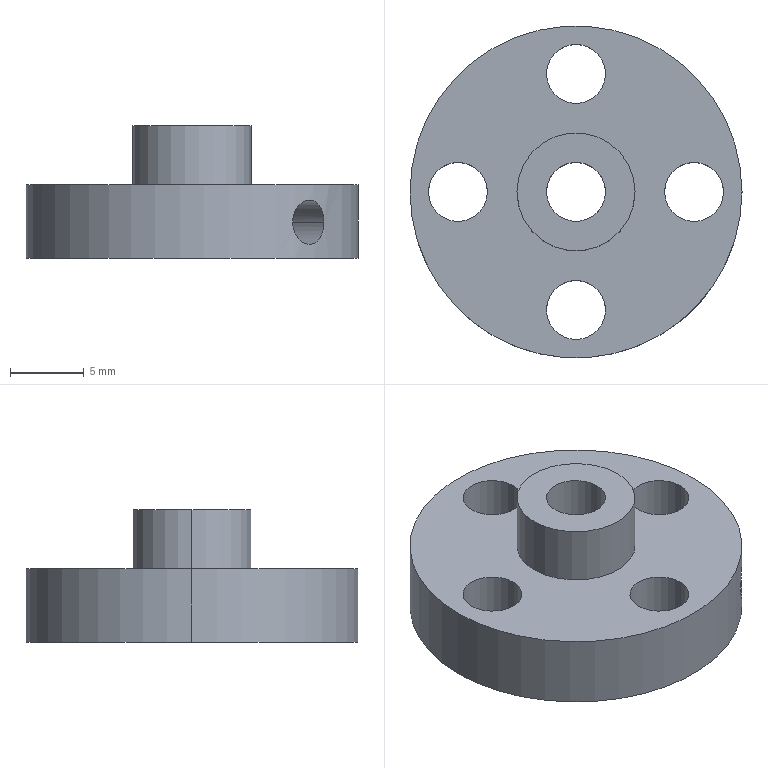Part | SolidWorks | features ICE 2, Extrusion 1 | 1 solid | 19 faces | box 22.5 x 22.5 x 9 mm | volume 1758 mm3 | cylinder 16 | plane 3 | commonest cylinder face diameters 4 x10 3 x2 8 x2 22.5 x2
STEP:
#1=CARTESIAN_POINT('',(2.,0.,1.958));
#2=VERTEX_POINT('',#1);
#3=CARTESIAN_POINT('',(-0.1252,-1.996,2.458));
#4=VERTEX_POINT('',#3);
#5=CARTESIAN_POINT('',(2.,0.,1.958));
#6=CARTESIAN_POINT('',(2.,-0.08244,1.793));
#7=CARTESIAN_POINT('',(1.995,-0.1967,1.645));
#8=CARTESIAN_POINT('',(1.952,-0.4524,1.385));
#9=CARTESIAN_POINT('',(1.915,-0.5972,1.271));
#10=CARTESIAN_POINT('',(1.797,-0.8915,1.091));
#11=CARTESIAN_POINT('',(1.714,-1.047,1.023));
#12=CARTESIAN_POINT('',(1.553,-1.264,0.9695));
#13=CARTESIAN_POINT('',(1.492,-1.335,0.9596));
#14=CARTESIAN_POINT('',(1.363,-1.466,0.9573));
#15=CARTESIAN_POINT('',(1.295,-1.527,0.9646));
#16=CARTESIAN_POINT('',(1.078,-1.694,1.011));
#17=CARTESIAN_POINT('',(0.9236,-1.781,1.075));
#18=CARTESIAN_POINT('',(0.6239,-1.907,1.251));
#19=CARTESIAN_POINT('',(0.4783,-1.946,1.363));
#20=CARTESIAN_POINT('',(0.2185,-1.992,1.619));
#21=CARTESIAN_POINT('',(0.1016,-1.999,1.766));
#22=CARTESIAN_POINT('',(-0.07068,-2.001,2.091));
#23=CARTESIAN_POINT('',(-0.1252,-1.996,2.273));
#24=CARTESIAN_POINT('',(-0.1252,-1.996,2.458));
#25=B_SPLINE_CURVE_WITH_KNOTS('',3,(#5,#6,#7,#8,#9,#10,#11,#12,#13,#14,#15,#16,#17,#18,#19,#20,#21,#22,#23,#24),.UNSPECIFIED.,.F.,.F.,(4,2,2,2,2,2,2,2,2,4),(0.0005162,0.001064,0.001612,0.00216,0.002434,0.002708,0.003256,0.003804,0.004352,0.004899),.UNSPECIFIED.);
#26=EDGE_CURVE('',#2,#4,#25,.T.);
#27=ORIENTED_EDGE('',*,*,#26,.T.);
#28=CARTESIAN_POINT('',(6.823,-8.945,2.458));
#29=VERTEX_POINT('',#28);
#30=CARTESIAN_POINT('',(-0.1768,-1.945,2.458));
#31=DIRECTION('',(0.7071,-0.7071,0.));
#32=VECTOR('',#31,1000.);
#33=LINE('',#30,#32);
#34=EDGE_CURVE('',#4,#29,#33,.T.);
#35=ORIENTED_EDGE('',*,*,#34,.T.);
#36=CARTESIAN_POINT('',(8.945,-6.823,2.458));
#37=VERTEX_POINT('',#36);
#38=CARTESIAN_POINT('',(8.945,-6.823,2.458));
#39=CARTESIAN_POINT('',(8.945,-6.823,2.359));
#40=CARTESIAN_POINT('',(8.939,-6.831,2.262));
#41=CARTESIAN_POINT('',(8.915,-6.862,2.07));
#42=CARTESIAN_POINT('',(8.897,-6.885,1.974));
#43=CARTESIAN_POINT('',(8.851,-6.945,1.793));
#44=CARTESIAN_POINT('',(8.822,-6.981,1.707));
#45=CARTESIAN_POINT('',(8.754,-7.067,1.544));
#46=CARTESIAN_POINT('',(8.714,-7.116,1.467));
#47=CARTESIAN_POINT('',(8.581,-7.277,1.259));
#48=CARTESIAN_POINT('',(8.472,-7.404,1.148));
#49=CARTESIAN_POINT('',(8.23,-7.672,0.9979));
#50=CARTESIAN_POINT('',(8.094,-7.816,0.9584));
#51=CARTESIAN_POINT('',(7.886,-8.024,0.9583));
#52=CARTESIAN_POINT('',(7.815,-8.093,0.9681));
#53=CARTESIAN_POINT('',(7.675,-8.226,1.006));
#54=CARTESIAN_POINT('',(7.606,-8.289,1.035));
#55=CARTESIAN_POINT('',(7.404,-8.472,1.148));
#56=CARTESIAN_POINT('',(7.278,-8.58,1.258));
#57=CARTESIAN_POINT('',(7.115,-8.714,1.468));
#58=CARTESIAN_POINT('',(7.067,-8.753,1.543));
#59=CARTESIAN_POINT('',(6.982,-8.822,1.706));
#60=CARTESIAN_POINT('',(6.944,-8.851,1.793));
#61=CARTESIAN_POINT('',(6.885,-8.898,1.975));
#62=CARTESIAN_POINT('',(6.862,-8.915,2.068));
#63=CARTESIAN_POINT('',(6.831,-8.939,2.261));
#64=CARTESIAN_POINT('',(6.823,-8.945,2.36));
#65=CARTESIAN_POINT('',(6.823,-8.945,2.458));
#66=B_SPLINE_CURVE_WITH_KNOTS('',3,(#38,#39,#40,#41,#42,#43,#44,#45,#46,#47,#48,#49,#50,#51,#52,#53,#54,#55,#56,#57,#58,#59,#60,#61,#62,#63,#64,#65),.UNSPECIFIED.,.F.,.F.,(4,2,2,2,2,2,2,2,2,2,2,2,2,4),(0.,0.0002934,0.0005869,0.0008803,0.001174,0.001761,0.002347,0.002641,0.002934,0.003521,0.003815,0.004108,0.004401,0.004695),.UNSPECIFIED.);
#67=EDGE_CURVE('',#37,#29,#66,.T.);
#68=ORIENTED_EDGE('',*,*,#67,.F.);
#69=CARTESIAN_POINT('',(1.996,0.1252,2.458));
#70=VERTEX_POINT('',#69);
#71=CARTESIAN_POINT('',(1.945,0.1768,2.458));
#72=DIRECTION('',(0.7071,-0.7071,0.));
#73=VECTOR('',#72,1000.);
#74=LINE('',#71,#73);
#75=EDGE_CURVE('',#70,#37,#74,.T.);
#76=ORIENTED_EDGE('',*,*,#75,.F.);
#77=CARTESIAN_POINT('',(1.996,0.1252,2.458));
#78=CARTESIAN_POINT('',(1.996,0.1252,2.371));
#79=CARTESIAN_POINT('',(1.997,0.1136,2.285));
#80=CARTESIAN_POINT('',(1.999,0.07067,2.118));
#81=CARTESIAN_POINT('',(2.,0.03884,2.036));
#82=CARTESIAN_POINT('',(2.,0.,1.958));
#83=B_SPLINE_CURVE_WITH_KNOTS('',3,(#77,#78,#79,#80,#81,#82),.UNSPECIFIED.,.F.,.F.,(4,2,4),(0.,0.0002581,0.0005162),.UNSPECIFIED.);
#84=EDGE_CURVE('',#70,#2,#83,.T.);
#85=ORIENTED_EDGE('',*,*,#84,.T.);
#86=EDGE_LOOP('',(#27,#35,#68,#76,#85));
#87=FACE_OUTER_BOUND('',#86,.T.);
#88=CARTESIAN_POINT('',(0.8839,-0.8839,2.458));
#89=DIRECTION('',(0.7071,-0.7071,0.));
#90=DIRECTION('',(0.7071,0.7071,0.));
#91=AXIS2_PLACEMENT_3D('',#88,#89,#90);
#92=CYLINDRICAL_SURFACE('',#91,1.5);
#93=ADVANCED_FACE('',(#87),#92,.F.);
#94=CARTESIAN_POINT('',(4.,0.,9.));
#95=VERTEX_POINT('',#94);
#96=CARTESIAN_POINT('',(-4.,0.,9.));
#97=VERTEX_POINT('',#96);
#98=CARTESIAN_POINT('',(0.,0.,9.));
#99=DIRECTION('',(0.,0.,1.));
#100=DIRECTION('',(1.,0.,0.));
#101=AXIS2_PLACEMENT_3D('',#98,#99,#100);
#102=CIRCLE('',#101,4.);
#103=EDGE_CURVE('',#95,#97,#102,.T.);
#104=ORIENTED_EDGE('',*,*,#103,.F.);
#105=CARTESIAN_POINT('',(4.,0.,5.));
#106=VERTEX_POINT('',#105);
#107=CARTESIAN_POINT('',(4.,0.,9.));
#108=DIRECTION('',(0.,0.,-1.));
#109=VECTOR('',#108,1000.);
#110=LINE('',#107,#109);
#111=EDGE_CURVE('',#95,#106,#110,.T.);
#112=ORIENTED_EDGE('',*,*,#111,.T.);
#113=CARTESIAN_POINT('',(-4.,0.,5.));
#114=VERTEX_POINT('',#113);
#115=CARTESIAN_POINT('',(0.,0.,5.));
#116=DIRECTION('',(0.,0.,1.));
#117=DIRECTION('',(1.,0.,0.));
#118=AXIS2_PLACEMENT_3D('',#115,#116,#117);
#119=CIRCLE('',#118,4.);
#120=EDGE_CURVE('',#106,#114,#119,.T.);
#121=ORIENTED_EDGE('',*,*,#120,.T.);
#122=CARTESIAN_POINT('',(-4.,0.,9.));
#123=DIRECTION('',(0.,0.,-1.));
#124=VECTOR('',#123,1000.);
#125=LINE('',#122,#124);
#126=EDGE_CURVE('',#97,#114,#125,.T.);
#127=ORIENTED_EDGE('',*,*,#126,.F.);
#128=EDGE_LOOP('',(#104,#112,#121,#127));
#129=FACE_OUTER_BOUND('',#128,.T.);
#130=CARTESIAN_POINT('',(0.,0.,9.));
#131=DIRECTION('',(0.,0.,-1.));
#132=DIRECTION('',(-1.,0.,0.));
#133=AXIS2_PLACEMENT_3D('',#130,#131,#132);
#134=CYLINDRICAL_SURFACE('',#133,4.);
#135=ADVANCED_FACE('',(#129),#134,.T.);
#136=CARTESIAN_POINT('',(6.,0.,5.));
#137=VERTEX_POINT('',#136);
#138=CARTESIAN_POINT('',(10.,0.,5.));
#139=VERTEX_POINT('',#138);
#140=CARTESIAN_POINT('',(8.,0.,5.));
#141=DIRECTION('',(0.,0.,1.));
#142=DIRECTION('',(1.,0.,0.));
#143=AXIS2_PLACEMENT_3D('',#140,#141,#142);
#144=CIRCLE('',#143,2.);
#145=EDGE_CURVE('',#137,#139,#144,.T.);
#146=ORIENTED_EDGE('',*,*,#145,.T.);
#147=CARTESIAN_POINT('',(10.,0.,0.));
#148=VERTEX_POINT('',#147);
#149=CARTESIAN_POINT('',(10.,0.,5.));
#150=DIRECTION('',(0.,0.,-1.));
#151=VECTOR('',#150,1000.);
#152=LINE('',#149,#151);
#153=EDGE_CURVE('',#139,#148,#152,.T.);
#154=ORIENTED_EDGE('',*,*,#153,.T.);
#155=CARTESIAN_POINT('',(6.,0.,0.));
#156=VERTEX_POINT('',#155);
#157=CARTESIAN_POINT('',(8.,0.,0.));
#158=DIRECTION('',(0.,0.,1.));
#159=DIRECTION('',(1.,0.,0.));
#160=AXIS2_PLACEMENT_3D('',#157,#158,#159);
#161=CIRCLE('',#160,2.);
#162=EDGE_CURVE('',#156,#148,#161,.T.);
#163=ORIENTED_EDGE('',*,*,#162,.F.);
#164=CARTESIAN_POINT('',(6.,0.,5.));
#165=DIRECTION('',(0.,0.,-1.));
#166=VECTOR('',#165,1000.);
#167=LINE('',#164,#166);
#168=EDGE_CURVE('',#137,#156,#167,.T.);
#169=ORIENTED_EDGE('',*,*,#168,.F.);
#170=EDGE_LOOP('',(#146,#154,#163,#169));
#171=FACE_OUTER_BOUND('',#170,.T.);
#172=CARTESIAN_POINT('',(8.,0.,5.));
#173=DIRECTION('',(0.,0.,-1.));
#174=DIRECTION('',(-1.,0.,0.));
#175=AXIS2_PLACEMENT_3D('',#172,#173,#174);
#176=CYLINDRICAL_SURFACE('',#175,2.);
#177=ADVANCED_FACE('',(#171),#176,.F.);
#178=CARTESIAN_POINT('',(-2.,0.,9.));
#179=VERTEX_POINT('',#178);
#180=CARTESIAN_POINT('',(2.,0.,9.));
#181=VERTEX_POINT('',#180);
#182=CARTESIAN_POINT('',(0.,0.,9.));
#183=DIRECTION('',(0.,0.,1.));
#184=DIRECTION('',(1.,0.,0.));
#185=AXIS2_PLACEMENT_3D('',#182,#183,#184);
#186=CIRCLE('',#185,2.);
#187=EDGE_CURVE('',#179,#181,#186,.T.);
#188=ORIENTED_EDGE('',*,*,#187,.T.);
#189=CARTESIAN_POINT('',(2.,0.,2.958));
#190=VERTEX_POINT('',#189);
#191=CARTESIAN_POINT('',(2.,0.,5.));
#192=DIRECTION('',(0.,0.,-1.));
#193=VECTOR('',#192,1000.);
#194=LINE('',#191,#193);
#195=EDGE_CURVE('',#181,#190,#194,.T.);
#196=ORIENTED_EDGE('',*,*,#195,.T.);
#197=CARTESIAN_POINT('',(-0.1252,-1.996,2.458));
#198=CARTESIAN_POINT('',(-0.1252,-1.996,2.644));
#199=CARTESIAN_POINT('',(-0.07048,-2.001,2.826));
#200=CARTESIAN_POINT('',(0.1014,-1.999,3.151));
#201=CARTESIAN_POINT('',(0.2181,-1.992,3.297));
#202=CARTESIAN_POINT('',(0.4776,-1.947,3.553));
#203=CARTESIAN_POINT('',(0.6235,-1.907,3.665));
#204=CARTESIAN_POINT('',(0.9189,-1.784,3.839));
#205=CARTESIAN_POINT('',(1.074,-1.697,3.904));
#206=CARTESIAN_POINT('',(1.289,-1.532,3.951));
#207=CARTESIAN_POINT('',(1.36,-1.47,3.959));
#208=CARTESIAN_POINT('',(1.489,-1.338,3.957));
#209=CARTESIAN_POINT('',(1.548,-1.269,3.948));
#210=CARTESIAN_POINT('',(1.712,-1.05,3.895));
#211=CARTESIAN_POINT('',(1.795,-0.8957,3.828));
#212=CARTESIAN_POINT('',(1.915,-0.5973,3.646));
#213=CARTESIAN_POINT('',(1.952,-0.4528,3.532));
#214=CARTESIAN_POINT('',(1.995,-0.1968,3.272));
#215=CARTESIAN_POINT('',(2.,-0.08225,3.123));
#216=CARTESIAN_POINT('',(2.,0.,2.958));
#217=B_SPLINE_CURVE_WITH_KNOTS('',3,(#197,#198,#199,#200,#201,#202,#203,#204,#205,#206,#207,#208,#209,#210,#211,#212,#213,#214,#215,#216),.UNSPECIFIED.,.F.,.F.,(4,2,2,2,2,2,2,2,2,4),(0.004899,0.005447,0.005994,0.006541,0.007088,0.007362,0.007635,0.008182,0.008729,0.009276),.UNSPECIFIED.);
#218=EDGE_CURVE('',#4,#190,#217,.T.);
#219=ORIENTED_EDGE('',*,*,#218,.F.);
#220=ORIENTED_EDGE('',*,*,#26,.F.);
#221=CARTESIAN_POINT('',(2.,0.,0.));
#222=VERTEX_POINT('',#221);
#223=CARTESIAN_POINT('',(2.,0.,5.));
#224=DIRECTION('',(0.,0.,-1.));
#225=VECTOR('',#224,1000.);
#226=LINE('',#223,#225);
#227=EDGE_CURVE('',#2,#222,#226,.T.);
#228=ORIENTED_EDGE('',*,*,#227,.T.);
#229=CARTESIAN_POINT('',(-2.,0.,0.));
#230=VERTEX_POINT('',#229);
#231=CARTESIAN_POINT('',(0.,0.,0.));
#232=DIRECTION('',(0.,0.,1.));
#233=DIRECTION('',(1.,0.,0.));
#234=AXIS2_PLACEMENT_3D('',#231,#232,#233);
#235=CIRCLE('',#234,2.);
#236=EDGE_CURVE('',#230,#222,#235,.T.);
#237=ORIENTED_EDGE('',*,*,#236,.F.);
#238=CARTESIAN_POINT('',(-2.,0.,5.));
#239=DIRECTION('',(0.,0.,-1.));
#240=VECTOR('',#239,1000.);
#241=LINE('',#238,#240);
#242=EDGE_CURVE('',#179,#230,#241,.T.);
#243=ORIENTED_EDGE('',*,*,#242,.F.);
#244=EDGE_LOOP('',(#188,#196,#219,#220,#228,#237,#243));
#245=FACE_OUTER_BOUND('',#244,.T.);
#246=CARTESIAN_POINT('',(0.,0.,5.));
#247=DIRECTION('',(0.,0.,-1.));
#248=DIRECTION('',(-1.,0.,0.));
#249=AXIS2_PLACEMENT_3D('',#246,#247,#248);
#250=CYLINDRICAL_SURFACE('',#249,2.);
#251=ADVANCED_FACE('',(#245),#250,.F.);
#252=CARTESIAN_POINT('',(-2.,8.,5.));
#253=VERTEX_POINT('',#252);
#254=CARTESIAN_POINT('',(2.,8.,5.));
#255=VERTEX_POINT('',#254);
#256=CARTESIAN_POINT('',(0.,8.,5.));
#257=DIRECTION('',(0.,0.,1.));
#258=DIRECTION('',(1.,0.,0.));
#259=AXIS2_PLACEMENT_3D('',#256,#257,#258);
#260=CIRCLE('',#259,2.);
#261=EDGE_CURVE('',#253,#255,#260,.T.);
#262=ORIENTED_EDGE('',*,*,#261,.T.);
#263=CARTESIAN_POINT('',(2.,8.,0.));
#264=VERTEX_POINT('',#263);
#265=CARTESIAN_POINT('',(2.,8.,5.));
#266=DIRECTION('',(0.,0.,-1.));
#267=VECTOR('',#266,1000.);
#268=LINE('',#265,#267);
#269=EDGE_CURVE('',#255,#264,#268,.T.);
#270=ORIENTED_EDGE('',*,*,#269,.T.);
#271=CARTESIAN_POINT('',(-2.,8.,0.));
#272=VERTEX_POINT('',#271);
#273=CARTESIAN_POINT('',(0.,8.,0.));
#274=DIRECTION('',(0.,0.,1.));
#275=DIRECTION('',(1.,0.,0.));
#276=AXIS2_PLACEMENT_3D('',#273,#274,#275);
#277=CIRCLE('',#276,2.);
#278=EDGE_CURVE('',#272,#264,#277,.T.);
#279=ORIENTED_EDGE('',*,*,#278,.F.);
#280=CARTESIAN_POINT('',(-2.,8.,5.));
#281=DIRECTION('',(0.,0.,-1.));
#282=VECTOR('',#281,1000.);
#283=LINE('',#280,#282);
#284=EDGE_CURVE('',#253,#272,#283,.T.);
#285=ORIENTED_EDGE('',*,*,#284,.F.);
#286=EDGE_LOOP('',(#262,#270,#279,#285));
#287=FACE_OUTER_BOUND('',#286,.T.);
#288=CARTESIAN_POINT('',(0.,8.,5.));
#289=DIRECTION('',(0.,0.,-1.));
#290=DIRECTION('',(-1.,0.,0.));
#291=AXIS2_PLACEMENT_3D('',#288,#289,#290);
#292=CYLINDRICAL_SURFACE('',#291,2.);
#293=ADVANCED_FACE('',(#287),#292,.F.);
#294=CARTESIAN_POINT('',(11.25,0.,5.));
#295=VERTEX_POINT('',#294);
#296=CARTESIAN_POINT('',(-11.25,0.,5.));
#297=VERTEX_POINT('',#296);
#298=CARTESIAN_POINT('',(0.,0.,5.));
#299=DIRECTION('',(0.,0.,1.));
#300=DIRECTION('',(1.,0.,0.));
#301=AXIS2_PLACEMENT_3D('',#298,#299,#300);
#302=CIRCLE('',#301,11.25);
#303=EDGE_CURVE('',#295,#297,#302,.T.);
#304=ORIENTED_EDGE('',*,*,#303,.F.);
#305=CARTESIAN_POINT('',(11.25,0.,0.));
#306=VERTEX_POINT('',#305);
#307=CARTESIAN_POINT('',(11.25,0.,5.));
#308=DIRECTION('',(0.,0.,-1.));
#309=VECTOR('',#308,1000.);
#310=LINE('',#307,#309);
#311=EDGE_CURVE('',#295,#306,#310,.T.);
#312=ORIENTED_EDGE('',*,*,#311,.T.);
#313=CARTESIAN_POINT('',(-11.25,0.,0.));
#314=VERTEX_POINT('',#313);
#315=CARTESIAN_POINT('',(0.,0.,0.));
#316=DIRECTION('',(0.,0.,1.));
#317=DIRECTION('',(1.,0.,0.));
#318=AXIS2_PLACEMENT_3D('',#315,#316,#317);
#319=CIRCLE('',#318,11.25);
#320=EDGE_CURVE('',#306,#314,#319,.T.);
#321=ORIENTED_EDGE('',*,*,#320,.T.);
#322=CARTESIAN_POINT('',(-11.25,0.,5.));
#323=DIRECTION('',(0.,0.,-1.));
#324=VECTOR('',#323,1000.);
#325=LINE('',#322,#324);
#326=EDGE_CURVE('',#297,#314,#325,.T.);
#327=ORIENTED_EDGE('',*,*,#326,.F.);
#328=EDGE_LOOP('',(#304,#312,#321,#327));
#329=FACE_OUTER_BOUND('',#328,.T.);
#330=CARTESIAN_POINT('',(0.,0.,5.));
#331=DIRECTION('',(0.,0.,-1.));
#332=DIRECTION('',(-1.,0.,0.));
#333=AXIS2_PLACEMENT_3D('',#330,#331,#332);
#334=CYLINDRICAL_SURFACE('',#333,11.25);
#335=ADVANCED_FACE('',(#329),#334,.T.);
#336=CARTESIAN_POINT('',(-10.,0.,5.));
#337=VERTEX_POINT('',#336);
#338=CARTESIAN_POINT('',(-6.,0.,5.));
#339=VERTEX_POINT('',#338);
#340=CARTESIAN_POINT('',(-8.,0.,5.));
#341=DIRECTION('',(0.,0.,1.));
#342=DIRECTION('',(1.,0.,0.));
#343=AXIS2_PLACEMENT_3D('',#340,#341,#342);
#344=CIRCLE('',#343,2.);
#345=EDGE_CURVE('',#337,#339,#344,.T.);
#346=ORIENTED_EDGE('',*,*,#345,.T.);
#347=CARTESIAN_POINT('',(-6.,0.,0.));
#348=VERTEX_POINT('',#347);
#349=CARTESIAN_POINT('',(-6.,0.,5.));
#350=DIRECTION('',(0.,0.,-1.));
#351=VECTOR('',#350,1000.);
#352=LINE('',#349,#351);
#353=EDGE_CURVE('',#339,#348,#352,.T.);
#354=ORIENTED_EDGE('',*,*,#353,.T.);
#355=CARTESIAN_POINT('',(-10.,0.,0.));
#356=VERTEX_POINT('',#355);
#357=CARTESIAN_POINT('',(-8.,0.,0.));
#358=DIRECTION('',(0.,0.,1.));
#359=DIRECTION('',(1.,0.,0.));
#360=AXIS2_PLACEMENT_3D('',#357,#358,#359);
#361=CIRCLE('',#360,2.);
#362=EDGE_CURVE('',#356,#348,#361,.T.);
#363=ORIENTED_EDGE('',*,*,#362,.F.);
#364=CARTESIAN_POINT('',(-10.,0.,5.));
#365=DIRECTION('',(0.,0.,-1.));
#366=VECTOR('',#365,1000.);
#367=LINE('',#364,#366);
#368=EDGE_CURVE('',#337,#356,#367,.T.);
#369=ORIENTED_EDGE('',*,*,#368,.F.);
#370=EDGE_LOOP('',(#346,#354,#363,#369));
#371=FACE_OUTER_BOUND('',#370,.T.);
#372=CARTESIAN_POINT('',(-8.,0.,5.));
#373=DIRECTION('',(0.,0.,-1.));
#374=DIRECTION('',(-1.,0.,0.));
#375=AXIS2_PLACEMENT_3D('',#372,#373,#374);
#376=CYLINDRICAL_SURFACE('',#375,2.);
#377=ADVANCED_FACE('',(#371),#376,.F.);
#378=CARTESIAN_POINT('',(-2.,-8.,5.));
#379=VERTEX_POINT('',#378);
#380=CARTESIAN_POINT('',(2.,-8.,5.));
#381=VERTEX_POINT('',#380);
#382=CARTESIAN_POINT('',(0.,-8.,5.));
#383=DIRECTION('',(0.,0.,1.));
#384=DIRECTION('',(1.,0.,0.));
#385=AXIS2_PLACEMENT_3D('',#382,#383,#384);
#386=CIRCLE('',#385,2.);
#387=EDGE_CURVE('',#379,#381,#386,.T.);
#388=ORIENTED_EDGE('',*,*,#387,.T.);
#389=CARTESIAN_POINT('',(2.,-8.,0.));
#390=VERTEX_POINT('',#389);
#391=CARTESIAN_POINT('',(2.,-8.,5.));
#392=DIRECTION('',(0.,0.,-1.));
#393=VECTOR('',#392,1000.);
#394=LINE('',#391,#393);
#395=EDGE_CURVE('',#381,#390,#394,.T.);
#396=ORIENTED_EDGE('',*,*,#395,.T.);
#397=CARTESIAN_POINT('',(-2.,-8.,0.));
#398=VERTEX_POINT('',#397);
#399=CARTESIAN_POINT('',(0.,-8.,0.));
#400=DIRECTION('',(0.,0.,1.));
#401=DIRECTION('',(1.,0.,0.));
#402=AXIS2_PLACEMENT_3D('',#399,#400,#401);
#403=CIRCLE('',#402,2.);
#404=EDGE_CURVE('',#398,#390,#403,.T.);
#405=ORIENTED_EDGE('',*,*,#404,.F.);
#406=CARTESIAN_POINT('',(-2.,-8.,5.));
#407=DIRECTION('',(0.,0.,-1.));
#408=VECTOR('',#407,1000.);
#409=LINE('',#406,#408);
#410=EDGE_CURVE('',#379,#398,#409,.T.);
#411=ORIENTED_EDGE('',*,*,#410,.F.);
#412=EDGE_LOOP('',(#388,#396,#405,#411));
#413=FACE_OUTER_BOUND('',#412,.T.);
#414=CARTESIAN_POINT('',(0.,-8.,5.));
#415=DIRECTION('',(0.,0.,-1.));
#416=DIRECTION('',(-1.,0.,0.));
#417=AXIS2_PLACEMENT_3D('',#414,#415,#416);
#418=CYLINDRICAL_SURFACE('',#417,2.);
#419=ADVANCED_FACE('',(#413),#418,.F.);
#420=ORIENTED_EDGE('',*,*,#145,.F.);
#421=CARTESIAN_POINT('',(8.,0.,5.));
#422=DIRECTION('',(0.,0.,1.));
#423=DIRECTION('',(1.,0.,0.));
#424=AXIS2_PLACEMENT_3D('',#421,#422,#423);
#425=CIRCLE('',#424,2.);
#426=EDGE_CURVE('',#139,#137,#425,.T.);
#427=ORIENTED_EDGE('',*,*,#426,.F.);
#428=EDGE_LOOP('',(#420,#427));
#429=FACE_BOUND('',#428,.T.);
#430=ORIENTED_EDGE('',*,*,#387,.F.);
#431=CARTESIAN_POINT('',(0.,-8.,5.));
#432=DIRECTION('',(0.,0.,1.));
#433=DIRECTION('',(1.,0.,0.));
#434=AXIS2_PLACEMENT_3D('',#431,#432,#433);
#435=CIRCLE('',#434,2.);
#436=EDGE_CURVE('',#381,#379,#435,.T.);
#437=ORIENTED_EDGE('',*,*,#436,.F.);
#438=EDGE_LOOP('',(#430,#437));
#439=FACE_BOUND('',#438,.T.);
#440=ORIENTED_EDGE('',*,*,#345,.F.);
#441=CARTESIAN_POINT('',(-8.,0.,5.));
#442=DIRECTION('',(0.,0.,1.));
#443=DIRECTION('',(1.,0.,0.));
#444=AXIS2_PLACEMENT_3D('',#441,#442,#443);
#445=CIRCLE('',#444,2.);
#446=EDGE_CURVE('',#339,#337,#445,.T.);
#447=ORIENTED_EDGE('',*,*,#446,.F.);
#448=EDGE_LOOP('',(#440,#447));
#449=FACE_BOUND('',#448,.T.);
#450=CARTESIAN_POINT('',(0.,0.,5.));
#451=DIRECTION('',(0.,0.,1.));
#452=DIRECTION('',(1.,0.,0.));
#453=AXIS2_PLACEMENT_3D('',#450,#451,#452);
#454=CIRCLE('',#453,11.25);
#455=EDGE_CURVE('',#297,#295,#454,.T.);
#456=ORIENTED_EDGE('',*,*,#455,.T.);
#457=ORIENTED_EDGE('',*,*,#303,.T.);
#458=EDGE_LOOP('',(#456,#457));
#459=FACE_OUTER_BOUND('',#458,.T.);
#460=ORIENTED_EDGE('',*,*,#261,.F.);
#461=CARTESIAN_POINT('',(0.,8.,5.));
#462=DIRECTION('',(0.,0.,1.));
#463=DIRECTION('',(1.,0.,0.));
#464=AXIS2_PLACEMENT_3D('',#461,#462,#463);
#465=CIRCLE('',#464,2.);
#466=EDGE_CURVE('',#255,#253,#465,.T.);
#467=ORIENTED_EDGE('',*,*,#466,.F.);
#468=EDGE_LOOP('',(#460,#467));
#469=FACE_BOUND('',#468,.T.);
#470=CARTESIAN_POINT('',(0.,0.,5.));
#471=DIRECTION('',(0.,0.,1.));
#472=DIRECTION('',(1.,0.,0.));
#473=AXIS2_PLACEMENT_3D('',#470,#471,#472);
#474=CIRCLE('',#473,4.);
#475=EDGE_CURVE('',#114,#106,#474,.T.);
#476=ORIENTED_EDGE('',*,*,#475,.F.);
#477=ORIENTED_EDGE('',*,*,#120,.F.);
#478=EDGE_LOOP('',(#476,#477));
#479=FACE_BOUND('',#478,.T.);
#480=CARTESIAN_POINT('',(0.,0.,5.));
#481=DIRECTION('',(0.,0.,1.));
#482=DIRECTION('',(1.,0.,0.));
#483=AXIS2_PLACEMENT_3D('',#480,#481,#482);
#484=PLANE('',#483);
#485=ADVANCED_FACE('',(#429,#439,#449,#459,#469,#479),#484,.T.);
#486=ORIENTED_EDGE('',*,*,#395,.F.);
#487=ORIENTED_EDGE('',*,*,#436,.T.);
#488=ORIENTED_EDGE('',*,*,#410,.T.);
#489=CARTESIAN_POINT('',(0.,-8.,0.));
#490=DIRECTION('',(0.,0.,1.));
#491=DIRECTION('',(1.,0.,0.));
#492=AXIS2_PLACEMENT_3D('',#489,#490,#491);
#493=CIRCLE('',#492,2.);
#494=EDGE_CURVE('',#390,#398,#493,.T.);
#495=ORIENTED_EDGE('',*,*,#494,.F.);
#496=EDGE_LOOP('',(#486,#487,#488,#495));
#497=FACE_OUTER_BOUND('',#496,.T.);
#498=CARTESIAN_POINT('',(0.,-8.,5.));
#499=DIRECTION('',(0.,0.,-1.));
#500=DIRECTION('',(-1.,0.,0.));
#501=AXIS2_PLACEMENT_3D('',#498,#499,#500);
#502=CYLINDRICAL_SURFACE('',#501,2.);
#503=ADVANCED_FACE('',(#497),#502,.F.);
#504=ORIENTED_EDGE('',*,*,#353,.F.);
#505=ORIENTED_EDGE('',*,*,#446,.T.);
#506=ORIENTED_EDGE('',*,*,#368,.T.);
#507=CARTESIAN_POINT('',(-8.,0.,0.));
#508=DIRECTION('',(0.,0.,1.));
#509=DIRECTION('',(1.,0.,0.));
#510=AXIS2_PLACEMENT_3D('',#507,#508,#509);
#511=CIRCLE('',#510,2.);
#512=EDGE_CURVE('',#348,#356,#511,.T.);
#513=ORIENTED_EDGE('',*,*,#512,.F.);
#514=EDGE_LOOP('',(#504,#505,#506,#513));
#515=FACE_OUTER_BOUND('',#514,.T.);
#516=CARTESIAN_POINT('',(-8.,0.,5.));
#517=DIRECTION('',(0.,0.,-1.));
#518=DIRECTION('',(-1.,0.,0.));
#519=AXIS2_PLACEMENT_3D('',#516,#517,#518);
#520=CYLINDRICAL_SURFACE('',#519,2.);
#521=ADVANCED_FACE('',(#515),#520,.F.);
#522=ORIENTED_EDGE('',*,*,#311,.F.);
#523=ORIENTED_EDGE('',*,*,#455,.F.);
#524=ORIENTED_EDGE('',*,*,#326,.T.);
#525=CARTESIAN_POINT('',(0.,0.,0.));
#526=DIRECTION('',(0.,0.,1.));
#527=DIRECTION('',(1.,0.,0.));
#528=AXIS2_PLACEMENT_3D('',#525,#526,#527);
#529=CIRCLE('',#528,11.25);
#530=EDGE_CURVE('',#314,#306,#529,.T.);
#531=ORIENTED_EDGE('',*,*,#530,.T.);
#532=EDGE_LOOP('',(#522,#523,#524,#531));
#533=FACE_OUTER_BOUND('',#532,.T.);
#534=ORIENTED_EDGE('',*,*,#67,.T.);
#535=CARTESIAN_POINT('',(6.823,-8.945,2.458));
#536=CARTESIAN_POINT('',(6.823,-8.945,2.654));
#537=CARTESIAN_POINT('',(6.855,-8.921,2.852));
#538=CARTESIAN_POINT('',(6.974,-8.828,3.213));
#539=CARTESIAN_POINT('',(7.062,-8.758,3.38));
#540=CARTESIAN_POINT('',(7.222,-8.626,3.587));
#541=CARTESIAN_POINT('',(7.282,-8.576,3.651));
#542=CARTESIAN_POINT('',(7.405,-8.469,3.76));
#543=CARTESIAN_POINT('',(7.47,-8.412,3.806));
#544=CARTESIAN_POINT('',(7.605,-8.291,3.881));
#545=CARTESIAN_POINT('',(7.675,-8.226,3.91));
#546=CARTESIAN_POINT('',(7.814,-8.094,3.948));
#547=CARTESIAN_POINT('',(7.884,-8.026,3.958));
#548=CARTESIAN_POINT('',(8.024,-7.886,3.958));
#549=CARTESIAN_POINT('',(8.092,-7.816,3.949));
#550=CARTESIAN_POINT('',(8.225,-7.676,3.911));
#551=CARTESIAN_POINT('',(8.289,-7.606,3.882));
#552=CARTESIAN_POINT('',(8.411,-7.471,3.807));
#553=CARTESIAN_POINT('',(8.468,-7.407,3.761));
#554=CARTESIAN_POINT('',(8.575,-7.283,3.652));
#555=CARTESIAN_POINT('',(8.625,-7.224,3.589));
#556=CARTESIAN_POINT('',(8.758,-7.063,3.382));
#557=CARTESIAN_POINT('',(8.827,-6.975,3.215));
#558=CARTESIAN_POINT('',(8.92,-6.855,2.854));
#559=CARTESIAN_POINT('',(8.945,-6.823,2.657));
#560=CARTESIAN_POINT('',(8.945,-6.823,2.458));
#561=B_SPLINE_CURVE_WITH_KNOTS('',3,(#535,#536,#537,#538,#539,#540,#541,#542,#543,#544,#545,#546,#547,#548,#549,#550,#551,#552,#553,#554,#555,#556,#557,#558,#559,#560),.UNSPECIFIED.,.F.,.F.,(4,2,2,2,2,2,2,2,2,2,2,2,4),(0.004695,0.005282,0.005868,0.006162,0.006455,0.006748,0.007042,0.007335,0.007629,0.007922,0.008215,0.008802,0.009389),.UNSPECIFIED.);
#562=EDGE_CURVE('',#29,#37,#561,.T.);
#563=ORIENTED_EDGE('',*,*,#562,.T.);
#564=EDGE_LOOP('',(#534,#563));
#565=FACE_BOUND('',#564,.T.);
#566=CARTESIAN_POINT('',(0.,0.,5.));
#567=DIRECTION('',(0.,0.,-1.));
#568=DIRECTION('',(-1.,0.,0.));
#569=AXIS2_PLACEMENT_3D('',#566,#567,#568);
#570=CYLINDRICAL_SURFACE('',#569,11.25);
#571=ADVANCED_FACE('',(#533,#565),#570,.T.);
#572=ORIENTED_EDGE('',*,*,#269,.F.);
#573=ORIENTED_EDGE('',*,*,#466,.T.);
#574=ORIENTED_EDGE('',*,*,#284,.T.);
#575=CARTESIAN_POINT('',(0.,8.,0.));
#576=DIRECTION('',(0.,0.,1.));
#577=DIRECTION('',(1.,0.,0.));
#578=AXIS2_PLACEMENT_3D('',#575,#576,#577);
#579=CIRCLE('',#578,2.);
#580=EDGE_CURVE('',#264,#272,#579,.T.);
#581=ORIENTED_EDGE('',*,*,#580,.F.);
#582=EDGE_LOOP('',(#572,#573,#574,#581));
#583=FACE_OUTER_BOUND('',#582,.T.);
#584=CARTESIAN_POINT('',(0.,8.,5.));
#585=DIRECTION('',(0.,0.,-1.));
#586=DIRECTION('',(-1.,0.,0.));
#587=AXIS2_PLACEMENT_3D('',#584,#585,#586);
#588=CYLINDRICAL_SURFACE('',#587,2.);
#589=ADVANCED_FACE('',(#583),#588,.F.);
#590=ORIENTED_EDGE('',*,*,#195,.F.);
#591=CARTESIAN_POINT('',(0.,0.,9.));
#592=DIRECTION('',(0.,0.,1.));
#593=DIRECTION('',(1.,0.,0.));
#594=AXIS2_PLACEMENT_3D('',#591,#592,#593);
#595=CIRCLE('',#594,2.);
#596=EDGE_CURVE('',#181,#179,#595,.T.);
#597=ORIENTED_EDGE('',*,*,#596,.T.);
#598=ORIENTED_EDGE('',*,*,#242,.T.);
#599=CARTESIAN_POINT('',(0.,0.,0.));
#600=DIRECTION('',(0.,0.,1.));
#601=DIRECTION('',(1.,0.,0.));
#602=AXIS2_PLACEMENT_3D('',#599,#600,#601);
#603=CIRCLE('',#602,2.);
#604=EDGE_CURVE('',#222,#230,#603,.T.);
#605=ORIENTED_EDGE('',*,*,#604,.F.);
#606=ORIENTED_EDGE('',*,*,#227,.F.);
#607=ORIENTED_EDGE('',*,*,#84,.F.);
#608=CARTESIAN_POINT('',(2.,0.,2.958));
#609=CARTESIAN_POINT('',(2.,0.03854,2.881));
#610=CARTESIAN_POINT('',(1.999,0.07022,2.8));
#611=CARTESIAN_POINT('',(1.997,0.1137,2.632));
#612=CARTESIAN_POINT('',(1.996,0.1252,2.546));
#613=CARTESIAN_POINT('',(1.996,0.1252,2.458));
#614=B_SPLINE_CURVE_WITH_KNOTS('',3,(#608,#609,#610,#611,#612,#613),.UNSPECIFIED.,.F.,.F.,(4,2,4),(0.009276,0.009533,0.009789),.UNSPECIFIED.);
#615=EDGE_CURVE('',#190,#70,#614,.T.);
#616=ORIENTED_EDGE('',*,*,#615,.F.);
#617=EDGE_LOOP('',(#590,#597,#598,#605,#606,#607,#616));
#618=FACE_OUTER_BOUND('',#617,.T.);
#619=CARTESIAN_POINT('',(0.,0.,5.));
#620=DIRECTION('',(0.,0.,-1.));
#621=DIRECTION('',(-1.,0.,0.));
#622=AXIS2_PLACEMENT_3D('',#619,#620,#621);
#623=CYLINDRICAL_SURFACE('',#622,2.);
#624=ADVANCED_FACE('',(#618),#623,.F.);
#625=ORIENTED_EDGE('',*,*,#153,.F.);
#626=ORIENTED_EDGE('',*,*,#426,.T.);
#627=ORIENTED_EDGE('',*,*,#168,.T.);
#628=CARTESIAN_POINT('',(8.,0.,0.));
#629=DIRECTION('',(0.,0.,1.));
#630=DIRECTION('',(1.,0.,0.));
#631=AXIS2_PLACEMENT_3D('',#628,#629,#630);
#632=CIRCLE('',#631,2.);
#633=EDGE_CURVE('',#148,#156,#632,.T.);
#634=ORIENTED_EDGE('',*,*,#633,.F.);
#635=EDGE_LOOP('',(#625,#626,#627,#634));
#636=FACE_OUTER_BOUND('',#635,.T.);
#637=CARTESIAN_POINT('',(8.,0.,5.));
#638=DIRECTION('',(0.,0.,-1.));
#639=DIRECTION('',(-1.,0.,0.));
#640=AXIS2_PLACEMENT_3D('',#637,#638,#639);
#641=CYLINDRICAL_SURFACE('',#640,2.);
#642=ADVANCED_FACE('',(#636),#641,.F.);
#643=ORIENTED_EDGE('',*,*,#236,.T.);
#644=ORIENTED_EDGE('',*,*,#604,.T.);
#645=EDGE_LOOP('',(#643,#644));
#646=FACE_BOUND('',#645,.T.);
#647=ORIENTED_EDGE('',*,*,#278,.T.);
#648=ORIENTED_EDGE('',*,*,#580,.T.);
#649=EDGE_LOOP('',(#647,#648));
#650=FACE_BOUND('',#649,.T.);
#651=ORIENTED_EDGE('',*,*,#530,.F.);
#652=ORIENTED_EDGE('',*,*,#320,.F.);
#653=EDGE_LOOP('',(#651,#652));
#654=FACE_OUTER_BOUND('',#653,.T.);
#655=ORIENTED_EDGE('',*,*,#362,.T.);
#656=ORIENTED_EDGE('',*,*,#512,.T.);
#657=EDGE_LOOP('',(#655,#656));
#658=FACE_BOUND('',#657,.T.);
#659=ORIENTED_EDGE('',*,*,#404,.T.);
#660=ORIENTED_EDGE('',*,*,#494,.T.);
#661=EDGE_LOOP('',(#659,#660));
#662=FACE_BOUND('',#661,.T.);
#663=ORIENTED_EDGE('',*,*,#162,.T.);
#664=ORIENTED_EDGE('',*,*,#633,.T.);
#665=EDGE_LOOP('',(#663,#664));
#666=FACE_BOUND('',#665,.T.);
#667=CARTESIAN_POINT('',(0.,0.,0.));
#668=DIRECTION('',(0.,0.,1.));
#669=DIRECTION('',(1.,0.,0.));
#670=AXIS2_PLACEMENT_3D('',#667,#668,#669);
#671=PLANE('',#670);
#672=ADVANCED_FACE('',(#646,#650,#654,#658,#662,#666),#671,.F.);
#673=CARTESIAN_POINT('',(0.,0.,9.));
#674=DIRECTION('',(0.,0.,1.));
#675=DIRECTION('',(1.,0.,0.));
#676=AXIS2_PLACEMENT_3D('',#673,#674,#675);
#677=CIRCLE('',#676,4.);
#678=EDGE_CURVE('',#97,#95,#677,.T.);
#679=ORIENTED_EDGE('',*,*,#678,.T.);
#680=ORIENTED_EDGE('',*,*,#103,.T.);
#681=EDGE_LOOP('',(#679,#680));
#682=FACE_OUTER_BOUND('',#681,.T.);
#683=ORIENTED_EDGE('',*,*,#187,.F.);
#684=ORIENTED_EDGE('',*,*,#596,.F.);
#685=EDGE_LOOP('',(#683,#684));
#686=FACE_BOUND('',#685,.T.);
#687=CARTESIAN_POINT('',(0.,0.,9.));
#688=DIRECTION('',(0.,0.,1.));
#689=DIRECTION('',(1.,0.,0.));
#690=AXIS2_PLACEMENT_3D('',#687,#688,#689);
#691=PLANE('',#690);
#692=ADVANCED_FACE('',(#682,#686),#691,.T.);
#693=ORIENTED_EDGE('',*,*,#111,.F.);
#694=ORIENTED_EDGE('',*,*,#678,.F.);
#695=ORIENTED_EDGE('',*,*,#126,.T.);
#696=ORIENTED_EDGE('',*,*,#475,.T.);
#697=EDGE_LOOP('',(#693,#694,#695,#696));
#698=FACE_OUTER_BOUND('',#697,.T.);
#699=CARTESIAN_POINT('',(0.,0.,9.));
#700=DIRECTION('',(0.,0.,-1.));
#701=DIRECTION('',(-1.,0.,0.));
#702=AXIS2_PLACEMENT_3D('',#699,#700,#701);
#703=CYLINDRICAL_SURFACE('',#702,4.);
#704=ADVANCED_FACE('',(#698),#703,.T.);
#705=ORIENTED_EDGE('',*,*,#34,.F.);
#706=ORIENTED_EDGE('',*,*,#218,.T.);
#707=ORIENTED_EDGE('',*,*,#615,.T.);
#708=ORIENTED_EDGE('',*,*,#75,.T.);
#709=ORIENTED_EDGE('',*,*,#562,.F.);
#710=EDGE_LOOP('',(#705,#706,#707,#708,#709));
#711=FACE_OUTER_BOUND('',#710,.T.);
#712=CARTESIAN_POINT('',(0.8839,-0.8839,2.458));
#713=DIRECTION('',(0.7071,-0.7071,0.));
#714=DIRECTION('',(0.7071,0.7071,0.));
#715=AXIS2_PLACEMENT_3D('',#712,#713,#714);
#716=CYLINDRICAL_SURFACE('',#715,1.5);
#717=ADVANCED_FACE('',(#711),#716,.F.);
#718=CLOSED_SHELL('',(#93,#135,#177,#251,#293,#335,#377,#419,#485,#503,#521,#571,#589,#624,#642,#672,#692,#704,#717));
#719=MANIFOLD_SOLID_BREP('',#718);
#720=CARTESIAN_POINT('',(0.,0.,0.));
#721=DIRECTION('',(0.,0.,1.));
#722=DIRECTION('',(1.,0.,0.));
#723=AXIS2_PLACEMENT_3D('',#720,#721,#722);
#724=(LENGTH_UNIT()NAMED_UNIT(*)SI_UNIT(.MILLI.,.METRE.));
#725=UNCERTAINTY_MEASURE_WITH_UNIT(LENGTH_MEASURE(0.00001),#724,'','');
#726=(NAMED_UNIT(*)PLANE_ANGLE_UNIT()SI_UNIT($,.RADIAN.));
#727=(NAMED_UNIT(*)SI_UNIT($,.STERADIAN.)SOLID_ANGLE_UNIT());
#728=(GEOMETRIC_REPRESENTATION_CONTEXT(3)GLOBAL_UNCERTAINTY_ASSIGNED_CONTEXT((#725))GLOBAL_UNIT_ASSIGNED_CONTEXT((#724,#726,#727))REPRESENTATION_CONTEXT('',''));
#729=ADVANCED_BREP_SHAPE_REPRESENTATION('',(#719,#723),#728);